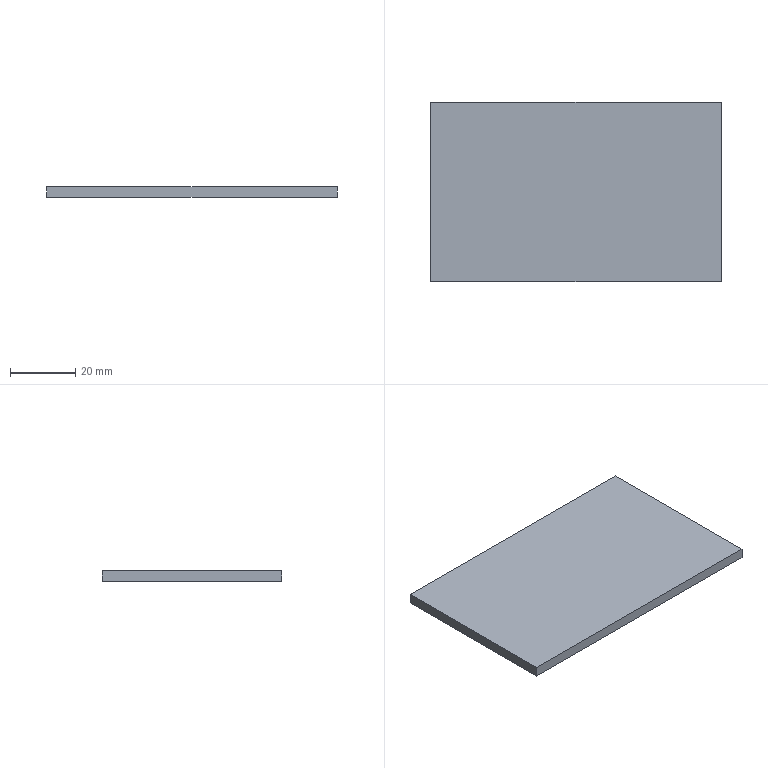Part | SolidWorks | features FlatPattern 1, SMBaseFlange 1, SheetMetal 1 | 1 solid | 6 faces | box 89 x 55 x 3.2 mm | volume 15664 mm3 | plane 6
STEP:
#1=CARTESIAN_POINT('',(44.5,-27.5,0.));
#2=VERTEX_POINT('',#1);
#3=CARTESIAN_POINT('',(44.5,27.5,0.));
#4=VERTEX_POINT('',#3);
#5=CARTESIAN_POINT('',(44.5,27.5,0.));
#6=DIRECTION('',(0.,1.,0.));
#7=VECTOR('',#6,1000.);
#8=LINE('',#5,#7);
#9=EDGE_CURVE('',#2,#4,#8,.T.);
#10=ORIENTED_EDGE('',*,*,#9,.T.);
#11=CARTESIAN_POINT('',(44.5,27.5,3.2));
#12=VERTEX_POINT('',#11);
#13=CARTESIAN_POINT('',(44.5,27.5,3.2));
#14=DIRECTION('',(0.,0.,-1.));
#15=VECTOR('',#14,1000.);
#16=LINE('',#13,#15);
#17=EDGE_CURVE('',#12,#4,#16,.T.);
#18=ORIENTED_EDGE('',*,*,#17,.F.);
#19=CARTESIAN_POINT('',(44.5,-27.5,3.2));
#20=VERTEX_POINT('',#19);
#21=CARTESIAN_POINT('',(44.5,27.5,3.2));
#22=DIRECTION('',(0.,1.,0.));
#23=VECTOR('',#22,1000.);
#24=LINE('',#21,#23);
#25=EDGE_CURVE('',#20,#12,#24,.T.);
#26=ORIENTED_EDGE('',*,*,#25,.F.);
#27=CARTESIAN_POINT('',(44.5,-27.5,3.2));
#28=DIRECTION('',(0.,0.,-1.));
#29=VECTOR('',#28,1000.);
#30=LINE('',#27,#29);
#31=EDGE_CURVE('',#20,#2,#30,.T.);
#32=ORIENTED_EDGE('',*,*,#31,.T.);
#33=EDGE_LOOP('',(#10,#18,#26,#32));
#34=FACE_OUTER_BOUND('',#33,.T.);
#35=CARTESIAN_POINT('',(44.5,27.5,3.2));
#36=DIRECTION('',(-1.,0.,0.));
#37=DIRECTION('',(0.,-1.,0.));
#38=AXIS2_PLACEMENT_3D('',#35,#36,#37);
#39=PLANE('',#38);
#40=ADVANCED_FACE('',(#34),#39,.F.);
#41=CARTESIAN_POINT('',(-44.5,27.5,0.));
#42=VERTEX_POINT('',#41);
#43=CARTESIAN_POINT('',(-44.5,27.5,0.));
#44=DIRECTION('',(-1.,0.,0.));
#45=VECTOR('',#44,1000.);
#46=LINE('',#43,#45);
#47=EDGE_CURVE('',#4,#42,#46,.T.);
#48=ORIENTED_EDGE('',*,*,#47,.T.);
#49=CARTESIAN_POINT('',(-44.5,27.5,3.2));
#50=VERTEX_POINT('',#49);
#51=CARTESIAN_POINT('',(-44.5,27.5,3.2));
#52=DIRECTION('',(0.,0.,-1.));
#53=VECTOR('',#52,1000.);
#54=LINE('',#51,#53);
#55=EDGE_CURVE('',#50,#42,#54,.T.);
#56=ORIENTED_EDGE('',*,*,#55,.F.);
#57=CARTESIAN_POINT('',(-44.5,27.5,3.2));
#58=DIRECTION('',(-1.,0.,0.));
#59=VECTOR('',#58,1000.);
#60=LINE('',#57,#59);
#61=EDGE_CURVE('',#12,#50,#60,.T.);
#62=ORIENTED_EDGE('',*,*,#61,.F.);
#63=ORIENTED_EDGE('',*,*,#17,.T.);
#64=EDGE_LOOP('',(#48,#56,#62,#63));
#65=FACE_OUTER_BOUND('',#64,.T.);
#66=CARTESIAN_POINT('',(-44.5,27.5,3.2));
#67=DIRECTION('',(0.,-1.,0.));
#68=DIRECTION('',(0.,0.,-1.));
#69=AXIS2_PLACEMENT_3D('',#66,#67,#68);
#70=PLANE('',#69);
#71=ADVANCED_FACE('',(#65),#70,.F.);
#72=CARTESIAN_POINT('',(-44.5,-27.5,0.));
#73=VERTEX_POINT('',#72);
#74=CARTESIAN_POINT('',(-44.5,27.5,0.));
#75=DIRECTION('',(0.,-1.,0.));
#76=VECTOR('',#75,1000.);
#77=LINE('',#74,#76);
#78=EDGE_CURVE('',#42,#73,#77,.T.);
#79=ORIENTED_EDGE('',*,*,#78,.T.);
#80=CARTESIAN_POINT('',(-44.5,-27.5,3.2));
#81=VERTEX_POINT('',#80);
#82=CARTESIAN_POINT('',(-44.5,-27.5,3.2));
#83=DIRECTION('',(0.,0.,-1.));
#84=VECTOR('',#83,1000.);
#85=LINE('',#82,#84);
#86=EDGE_CURVE('',#81,#73,#85,.T.);
#87=ORIENTED_EDGE('',*,*,#86,.F.);
#88=CARTESIAN_POINT('',(-44.5,27.5,3.2));
#89=DIRECTION('',(0.,-1.,0.));
#90=VECTOR('',#89,1000.);
#91=LINE('',#88,#90);
#92=EDGE_CURVE('',#50,#81,#91,.T.);
#93=ORIENTED_EDGE('',*,*,#92,.F.);
#94=ORIENTED_EDGE('',*,*,#55,.T.);
#95=EDGE_LOOP('',(#79,#87,#93,#94));
#96=FACE_OUTER_BOUND('',#95,.T.);
#97=CARTESIAN_POINT('',(-44.5,27.5,3.2));
#98=DIRECTION('',(1.,0.,0.));
#99=DIRECTION('',(0.,1.,0.));
#100=AXIS2_PLACEMENT_3D('',#97,#98,#99);
#101=PLANE('',#100);
#102=ADVANCED_FACE('',(#96),#101,.F.);
#103=CARTESIAN_POINT('',(-44.5,-27.5,0.));
#104=DIRECTION('',(1.,0.,0.));
#105=VECTOR('',#104,1000.);
#106=LINE('',#103,#105);
#107=EDGE_CURVE('',#73,#2,#106,.T.);
#108=ORIENTED_EDGE('',*,*,#107,.T.);
#109=ORIENTED_EDGE('',*,*,#31,.F.);
#110=CARTESIAN_POINT('',(-44.5,-27.5,3.2));
#111=DIRECTION('',(1.,0.,0.));
#112=VECTOR('',#111,1000.);
#113=LINE('',#110,#112);
#114=EDGE_CURVE('',#81,#20,#113,.T.);
#115=ORIENTED_EDGE('',*,*,#114,.F.);
#116=ORIENTED_EDGE('',*,*,#86,.T.);
#117=EDGE_LOOP('',(#108,#109,#115,#116));
#118=FACE_OUTER_BOUND('',#117,.T.);
#119=CARTESIAN_POINT('',(-44.5,-27.5,3.2));
#120=DIRECTION('',(0.,1.,0.));
#121=DIRECTION('',(0.,0.,1.));
#122=AXIS2_PLACEMENT_3D('',#119,#120,#121);
#123=PLANE('',#122);
#124=ADVANCED_FACE('',(#118),#123,.F.);
#125=ORIENTED_EDGE('',*,*,#25,.T.);
#126=ORIENTED_EDGE('',*,*,#61,.T.);
#127=ORIENTED_EDGE('',*,*,#92,.T.);
#128=ORIENTED_EDGE('',*,*,#114,.T.);
#129=EDGE_LOOP('',(#125,#126,#127,#128));
#130=FACE_OUTER_BOUND('',#129,.T.);
#131=CARTESIAN_POINT('',(0.,0.,3.2));
#132=DIRECTION('',(0.,0.,1.));
#133=DIRECTION('',(1.,0.,0.));
#134=AXIS2_PLACEMENT_3D('',#131,#132,#133);
#135=PLANE('',#134);
#136=ADVANCED_FACE('',(#130),#135,.T.);
#137=ORIENTED_EDGE('',*,*,#9,.F.);
#138=ORIENTED_EDGE('',*,*,#107,.F.);
#139=ORIENTED_EDGE('',*,*,#78,.F.);
#140=ORIENTED_EDGE('',*,*,#47,.F.);
#141=EDGE_LOOP('',(#137,#138,#139,#140));
#142=FACE_OUTER_BOUND('',#141,.T.);
#143=CARTESIAN_POINT('',(0.,0.,0.));
#144=DIRECTION('',(0.,0.,1.));
#145=DIRECTION('',(1.,0.,0.));
#146=AXIS2_PLACEMENT_3D('',#143,#144,#145);
#147=PLANE('',#146);
#148=ADVANCED_FACE('',(#142),#147,.F.);
#149=CLOSED_SHELL('',(#40,#71,#102,#124,#136,#148));
#150=MANIFOLD_SOLID_BREP('',#149);
#151=CARTESIAN_POINT('',(0.,0.,0.));
#152=DIRECTION('',(0.,0.,1.));
#153=DIRECTION('',(1.,0.,0.));
#154=AXIS2_PLACEMENT_3D('',#151,#152,#153);
#155=(LENGTH_UNIT()NAMED_UNIT(*)SI_UNIT(.MILLI.,.METRE.));
#156=UNCERTAINTY_MEASURE_WITH_UNIT(LENGTH_MEASURE(0.00001),#155,'','');
#157=(NAMED_UNIT(*)PLANE_ANGLE_UNIT()SI_UNIT($,.RADIAN.));
#158=(NAMED_UNIT(*)SI_UNIT($,.STERADIAN.)SOLID_ANGLE_UNIT());
#159=(GEOMETRIC_REPRESENTATION_CONTEXT(3)GLOBAL_UNCERTAINTY_ASSIGNED_CONTEXT((#156))GLOBAL_UNIT_ASSIGNED_CONTEXT((#155,#157,#158))REPRESENTATION_CONTEXT('',''));
#160=ADVANCED_BREP_SHAPE_REPRESENTATION('',(#150,#154),#159);